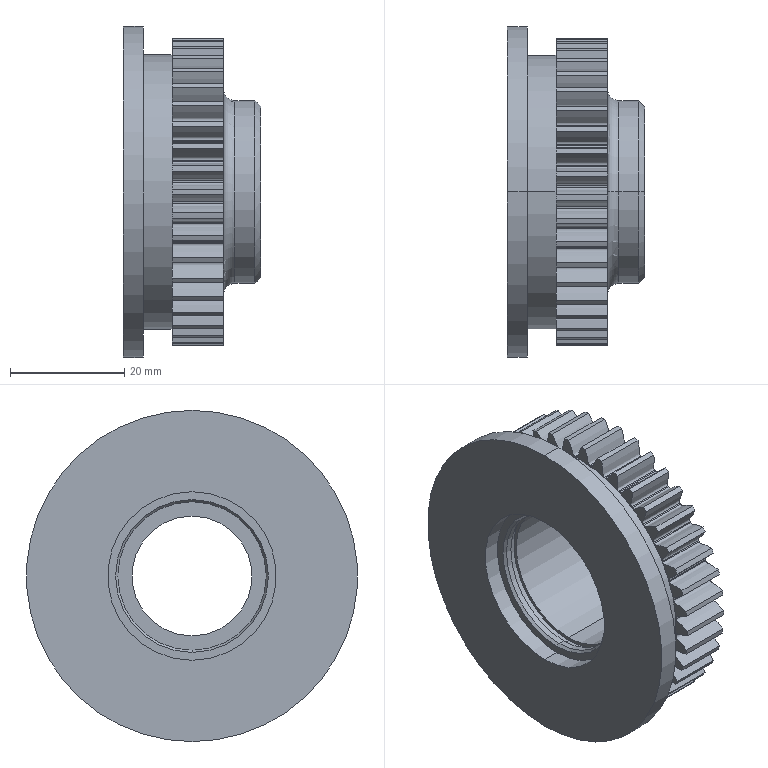Part | SolidWorks | features ICE 4, Chamfer 3, CirPattern 1, Extrusion 1, Fillet 1, RefAxis 1, RevCut 1 | 1 solid | 197 faces | box 24 x 58 x 58 mm | volume 29070 mm3 | cylinder 98 | spline 82 | plane 9 | cone 6 | torus 2 | commonest cylinder face diameters 48.125 x41 53.75 x41 26 x4 21 x2 27.2 x2 29.5 x2